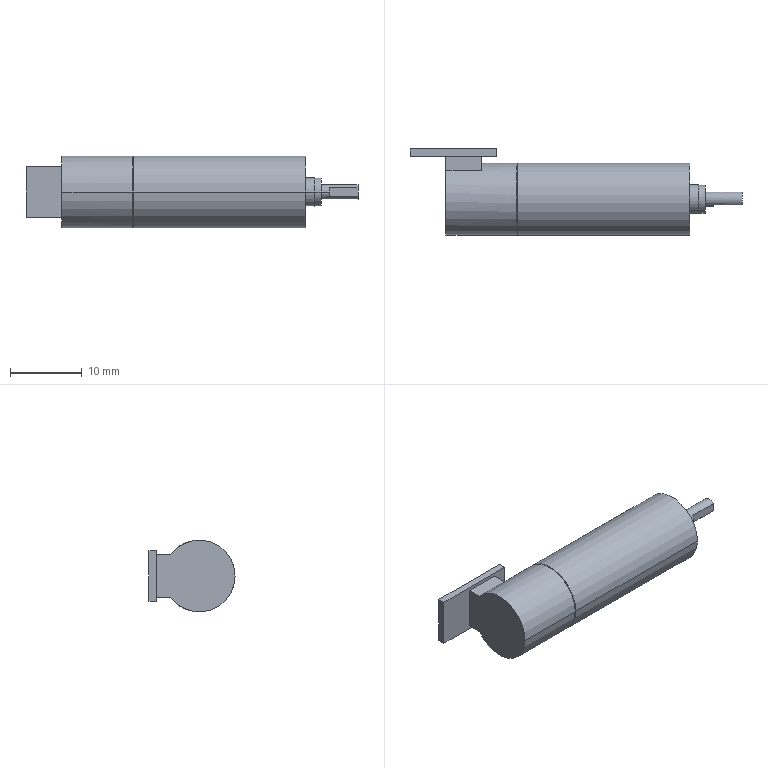Part | SolidWorks | features BaseBody 1 | 1 solid | 30 faces | box 46.3 x 12 x 10 mm | volume 2836 mm3 | plane 18 | cylinder 12 | commonest cylinder face diameters 10 x4 2 x2 3.9 x2 4 x2 9.8 x2
STEP:
#1=CARTESIAN_POINT('',(-31.3,5.,0.));
#2=VERTEX_POINT('',#1);
#3=CARTESIAN_POINT('',(-31.3,-5.,0.));
#4=VERTEX_POINT('',#3);
#5=CARTESIAN_POINT('',(-31.3,0.,0.));
#6=DIRECTION('',(1.,0.,0.));
#7=DIRECTION('',(0.,1.,0.));
#8=AXIS2_PLACEMENT_3D('',#5,#6,#7);
#9=CIRCLE('',#8,5.);
#10=EDGE_CURVE('',#2,#4,#9,.T.);
#11=ORIENTED_EDGE('',*,*,#10,.T.);
#12=CARTESIAN_POINT('',(-7.3,-5.,0.));
#13=VERTEX_POINT('',#12);
#14=CARTESIAN_POINT('',(0.,-5.,0.));
#15=DIRECTION('',(1.,0.,0.));
#16=VECTOR('',#15,1000.);
#17=LINE('',#14,#16);
#18=EDGE_CURVE('',#4,#13,#17,.T.);
#19=ORIENTED_EDGE('',*,*,#18,.T.);
#20=CARTESIAN_POINT('',(-7.3,5.,0.));
#21=VERTEX_POINT('',#20);
#22=CARTESIAN_POINT('',(-7.3,0.,0.));
#23=DIRECTION('',(-1.,0.,0.));
#24=DIRECTION('',(0.,1.,0.));
#25=AXIS2_PLACEMENT_3D('',#22,#23,#24);
#26=CIRCLE('',#25,5.);
#27=EDGE_CURVE('',#13,#21,#26,.T.);
#28=ORIENTED_EDGE('',*,*,#27,.T.);
#29=CARTESIAN_POINT('',(0.,5.,0.));
#30=DIRECTION('',(1.,0.,0.));
#31=VECTOR('',#30,1000.);
#32=LINE('',#29,#31);
#33=EDGE_CURVE('',#2,#21,#32,.T.);
#34=ORIENTED_EDGE('',*,*,#33,.F.);
#35=EDGE_LOOP('',(#11,#19,#28,#34));
#36=FACE_OUTER_BOUND('',#35,.T.);
#37=CARTESIAN_POINT('',(0.,0.,0.));
#38=DIRECTION('',(1.,0.,0.));
#39=DIRECTION('',(0.,1.,0.));
#40=AXIS2_PLACEMENT_3D('',#37,#38,#39);
#41=CYLINDRICAL_SURFACE('',#40,5.);
#42=ADVANCED_FACE('',(#36),#41,.T.);
#43=CARTESIAN_POINT('',(-7.3,-2.,0.));
#44=VERTEX_POINT('',#43);
#45=CARTESIAN_POINT('',(-7.3,2.,0.));
#46=VERTEX_POINT('',#45);
#47=CARTESIAN_POINT('',(-7.3,0.,0.));
#48=DIRECTION('',(-1.,0.,0.));
#49=DIRECTION('',(0.,1.,0.));
#50=AXIS2_PLACEMENT_3D('',#47,#48,#49);
#51=CIRCLE('',#50,2.);
#52=EDGE_CURVE('',#44,#46,#51,.T.);
#53=ORIENTED_EDGE('',*,*,#52,.F.);
#54=CARTESIAN_POINT('',(-6.02,-2.,0.));
#55=VERTEX_POINT('',#54);
#56=CARTESIAN_POINT('',(0.,-2.,0.));
#57=DIRECTION('',(1.,0.,0.));
#58=VECTOR('',#57,1000.);
#59=LINE('',#56,#58);
#60=EDGE_CURVE('',#44,#55,#59,.T.);
#61=ORIENTED_EDGE('',*,*,#60,.T.);
#62=CARTESIAN_POINT('',(-6.02,2.,0.));
#63=VERTEX_POINT('',#62);
#64=CARTESIAN_POINT('',(-6.02,0.,0.));
#65=DIRECTION('',(-1.,0.,0.));
#66=DIRECTION('',(0.,1.,0.));
#67=AXIS2_PLACEMENT_3D('',#64,#65,#66);
#68=CIRCLE('',#67,2.);
#69=EDGE_CURVE('',#55,#63,#68,.T.);
#70=ORIENTED_EDGE('',*,*,#69,.T.);
#71=CARTESIAN_POINT('',(0.,2.,0.));
#72=DIRECTION('',(1.,0.,0.));
#73=VECTOR('',#72,1000.);
#74=LINE('',#71,#73);
#75=EDGE_CURVE('',#46,#63,#74,.T.);
#76=ORIENTED_EDGE('',*,*,#75,.F.);
#77=EDGE_LOOP('',(#53,#61,#70,#76));
#78=FACE_OUTER_BOUND('',#77,.T.);
#79=CARTESIAN_POINT('',(0.,0.,0.));
#80=DIRECTION('',(1.,0.,0.));
#81=DIRECTION('',(0.,1.,0.));
#82=AXIS2_PLACEMENT_3D('',#79,#80,#81);
#83=CYLINDRICAL_SURFACE('',#82,2.);
#84=ADVANCED_FACE('',(#78),#83,.T.);
#85=CARTESIAN_POINT('',(-31.4,4.9,0.));
#86=VERTEX_POINT('',#85);
#87=CARTESIAN_POINT('',(-31.4,-4.9,0.));
#88=VERTEX_POINT('',#87);
#89=CARTESIAN_POINT('',(-31.4,0.,0.));
#90=DIRECTION('',(1.,0.,0.));
#91=DIRECTION('',(0.,1.,0.));
#92=AXIS2_PLACEMENT_3D('',#89,#90,#91);
#93=CIRCLE('',#92,4.9);
#94=EDGE_CURVE('',#86,#88,#93,.T.);
#95=ORIENTED_EDGE('',*,*,#94,.T.);
#96=CARTESIAN_POINT('',(-31.3,-4.9,0.));
#97=VERTEX_POINT('',#96);
#98=CARTESIAN_POINT('',(0.,-4.9,0.));
#99=DIRECTION('',(1.,0.,0.));
#100=VECTOR('',#99,1000.);
#101=LINE('',#98,#100);
#102=EDGE_CURVE('',#88,#97,#101,.T.);
#103=ORIENTED_EDGE('',*,*,#102,.T.);
#104=CARTESIAN_POINT('',(-31.3,4.9,0.));
#105=VERTEX_POINT('',#104);
#106=CARTESIAN_POINT('',(-31.3,0.,0.));
#107=DIRECTION('',(1.,0.,0.));
#108=DIRECTION('',(0.,1.,0.));
#109=AXIS2_PLACEMENT_3D('',#106,#107,#108);
#110=CIRCLE('',#109,4.9);
#111=EDGE_CURVE('',#105,#97,#110,.T.);
#112=ORIENTED_EDGE('',*,*,#111,.F.);
#113=CARTESIAN_POINT('',(0.,4.9,0.));
#114=DIRECTION('',(1.,0.,0.));
#115=VECTOR('',#114,1000.);
#116=LINE('',#113,#115);
#117=EDGE_CURVE('',#86,#105,#116,.T.);
#118=ORIENTED_EDGE('',*,*,#117,.F.);
#119=EDGE_LOOP('',(#95,#103,#112,#118));
#120=FACE_OUTER_BOUND('',#119,.T.);
#121=CARTESIAN_POINT('',(0.,0.,0.));
#122=DIRECTION('',(1.,0.,0.));
#123=DIRECTION('',(0.,1.,0.));
#124=AXIS2_PLACEMENT_3D('',#121,#122,#123);
#125=CYLINDRICAL_SURFACE('',#124,4.9);
#126=ADVANCED_FACE('',(#120),#125,.T.);
#127=CARTESIAN_POINT('',(-6.02,-1.95,0.));
#128=VERTEX_POINT('',#127);
#129=CARTESIAN_POINT('',(-6.02,1.95,0.));
#130=VERTEX_POINT('',#129);
#131=CARTESIAN_POINT('',(-6.02,0.,0.));
#132=DIRECTION('',(-1.,0.,0.));
#133=DIRECTION('',(0.,1.,0.));
#134=AXIS2_PLACEMENT_3D('',#131,#132,#133);
#135=CIRCLE('',#134,1.95);
#136=EDGE_CURVE('',#128,#130,#135,.T.);
#137=ORIENTED_EDGE('',*,*,#136,.F.);
#138=CARTESIAN_POINT('',(-5.14,-1.95,0.));
#139=VERTEX_POINT('',#138);
#140=CARTESIAN_POINT('',(0.,-1.95,0.));
#141=DIRECTION('',(1.,0.,0.));
#142=VECTOR('',#141,1000.);
#143=LINE('',#140,#142);
#144=EDGE_CURVE('',#128,#139,#143,.T.);
#145=ORIENTED_EDGE('',*,*,#144,.T.);
#146=CARTESIAN_POINT('',(-5.14,1.95,0.));
#147=VERTEX_POINT('',#146);
#148=CARTESIAN_POINT('',(-5.14,0.,0.));
#149=DIRECTION('',(-1.,0.,0.));
#150=DIRECTION('',(0.,1.,0.));
#151=AXIS2_PLACEMENT_3D('',#148,#149,#150);
#152=CIRCLE('',#151,1.95);
#153=EDGE_CURVE('',#139,#147,#152,.T.);
#154=ORIENTED_EDGE('',*,*,#153,.T.);
#155=CARTESIAN_POINT('',(0.,1.95,0.));
#156=DIRECTION('',(1.,0.,0.));
#157=VECTOR('',#156,1000.);
#158=LINE('',#155,#157);
#159=EDGE_CURVE('',#130,#147,#158,.T.);
#160=ORIENTED_EDGE('',*,*,#159,.F.);
#161=EDGE_LOOP('',(#137,#145,#154,#160));
#162=FACE_OUTER_BOUND('',#161,.T.);
#163=CARTESIAN_POINT('',(0.,0.,0.));
#164=DIRECTION('',(1.,0.,0.));
#165=DIRECTION('',(0.,1.,0.));
#166=AXIS2_PLACEMENT_3D('',#163,#164,#165);
#167=CYLINDRICAL_SURFACE('',#166,1.95);
#168=ADVANCED_FACE('',(#162),#167,.T.);
#169=CARTESIAN_POINT('',(-41.3,4.,3.));
#170=VERTEX_POINT('',#169);
#171=CARTESIAN_POINT('',(-41.3,-5.,0.));
#172=VERTEX_POINT('',#171);
#173=CARTESIAN_POINT('',(-41.3,0.,0.));
#174=DIRECTION('',(1.,0.,0.));
#175=DIRECTION('',(0.,1.,0.));
#176=AXIS2_PLACEMENT_3D('',#173,#174,#175);
#177=CIRCLE('',#176,5.);
#178=EDGE_CURVE('',#170,#172,#177,.T.);
#179=ORIENTED_EDGE('',*,*,#178,.T.);
#180=CARTESIAN_POINT('',(-31.4,-5.,0.));
#181=VERTEX_POINT('',#180);
#182=CARTESIAN_POINT('',(0.,-5.,0.));
#183=DIRECTION('',(1.,0.,0.));
#184=VECTOR('',#183,1000.);
#185=LINE('',#182,#184);
#186=EDGE_CURVE('',#172,#181,#185,.T.);
#187=ORIENTED_EDGE('',*,*,#186,.T.);
#188=CARTESIAN_POINT('',(-31.4,5.,0.));
#189=VERTEX_POINT('',#188);
#190=CARTESIAN_POINT('',(-31.4,0.,0.));
#191=DIRECTION('',(1.,0.,0.));
#192=DIRECTION('',(0.,1.,0.));
#193=AXIS2_PLACEMENT_3D('',#190,#191,#192);
#194=CIRCLE('',#193,5.);
#195=EDGE_CURVE('',#189,#181,#194,.T.);
#196=ORIENTED_EDGE('',*,*,#195,.F.);
#197=CARTESIAN_POINT('',(-36.3,5.,0.));
#198=VERTEX_POINT('',#197);
#199=CARTESIAN_POINT('',(0.,5.,0.));
#200=DIRECTION('',(1.,0.,0.));
#201=VECTOR('',#200,1000.);
#202=LINE('',#199,#201);
#203=EDGE_CURVE('',#198,#189,#202,.T.);
#204=ORIENTED_EDGE('',*,*,#203,.F.);
#205=CARTESIAN_POINT('',(-36.3,4.,3.));
#206=VERTEX_POINT('',#205);
#207=CARTESIAN_POINT('',(-36.3,0.,0.));
#208=DIRECTION('',(1.,0.,0.));
#209=DIRECTION('',(0.,1.,0.));
#210=AXIS2_PLACEMENT_3D('',#207,#208,#209);
#211=CIRCLE('',#210,5.);
#212=EDGE_CURVE('',#198,#206,#211,.T.);
#213=ORIENTED_EDGE('',*,*,#212,.T.);
#214=CARTESIAN_POINT('',(0.,4.,3.));
#215=DIRECTION('',(-1.,0.,0.));
#216=VECTOR('',#215,1000.);
#217=LINE('',#214,#216);
#218=EDGE_CURVE('',#206,#170,#217,.T.);
#219=ORIENTED_EDGE('',*,*,#218,.T.);
#220=EDGE_LOOP('',(#179,#187,#196,#204,#213,#219));
#221=FACE_OUTER_BOUND('',#220,.T.);
#222=CARTESIAN_POINT('',(0.,0.,0.));
#223=DIRECTION('',(1.,0.,0.));
#224=DIRECTION('',(0.,1.,0.));
#225=AXIS2_PLACEMENT_3D('',#222,#223,#224);
#226=CYLINDRICAL_SURFACE('',#225,5.);
#227=ADVANCED_FACE('',(#221),#226,.T.);
#228=CARTESIAN_POINT('',(-5.14,-1.,0.));
#229=VERTEX_POINT('',#228);
#230=CARTESIAN_POINT('',(-5.14,1.,0.));
#231=VERTEX_POINT('',#230);
#232=CARTESIAN_POINT('',(-5.14,0.,0.));
#233=DIRECTION('',(-1.,0.,0.));
#234=DIRECTION('',(0.,1.,0.));
#235=AXIS2_PLACEMENT_3D('',#232,#233,#234);
#236=CIRCLE('',#235,1.);
#237=EDGE_CURVE('',#229,#231,#236,.T.);
#238=ORIENTED_EDGE('',*,*,#237,.F.);
#239=CARTESIAN_POINT('',(-4.,-1.,0.));
#240=VERTEX_POINT('',#239);
#241=CARTESIAN_POINT('',(0.,-1.,0.));
#242=DIRECTION('',(1.,0.,0.));
#243=VECTOR('',#242,1000.);
#244=LINE('',#241,#243);
#245=EDGE_CURVE('',#229,#240,#244,.T.);
#246=ORIENTED_EDGE('',*,*,#245,.T.);
#247=CARTESIAN_POINT('',(-4.,-0.8,0.6));
#248=VERTEX_POINT('',#247);
#249=CARTESIAN_POINT('',(-4.,0.,0.));
#250=DIRECTION('',(-1.,0.,0.));
#251=DIRECTION('',(0.,1.,0.));
#252=AXIS2_PLACEMENT_3D('',#249,#250,#251);
#253=CIRCLE('',#252,1.);
#254=EDGE_CURVE('',#240,#248,#253,.T.);
#255=ORIENTED_EDGE('',*,*,#254,.T.);
#256=CARTESIAN_POINT('',(0.,-0.8,0.6));
#257=VERTEX_POINT('',#256);
#258=CARTESIAN_POINT('',(0.,-0.8,0.6));
#259=DIRECTION('',(1.,0.,0.));
#260=VECTOR('',#259,1000.);
#261=LINE('',#258,#260);
#262=EDGE_CURVE('',#248,#257,#261,.T.);
#263=ORIENTED_EDGE('',*,*,#262,.T.);
#264=CARTESIAN_POINT('',(0.,1.,0.));
#265=VERTEX_POINT('',#264);
#266=CARTESIAN_POINT('',(0.,0.,0.));
#267=DIRECTION('',(-1.,0.,0.));
#268=DIRECTION('',(0.,1.,0.));
#269=AXIS2_PLACEMENT_3D('',#266,#267,#268);
#270=CIRCLE('',#269,1.);
#271=EDGE_CURVE('',#257,#265,#270,.T.);
#272=ORIENTED_EDGE('',*,*,#271,.T.);
#273=CARTESIAN_POINT('',(0.,1.,0.));
#274=DIRECTION('',(1.,0.,0.));
#275=VECTOR('',#274,1000.);
#276=LINE('',#273,#275);
#277=EDGE_CURVE('',#231,#265,#276,.T.);
#278=ORIENTED_EDGE('',*,*,#277,.F.);
#279=EDGE_LOOP('',(#238,#246,#255,#263,#272,#278));
#280=FACE_OUTER_BOUND('',#279,.T.);
#281=CARTESIAN_POINT('',(0.,0.,0.));
#282=DIRECTION('',(1.,0.,0.));
#283=DIRECTION('',(0.,1.,0.));
#284=AXIS2_PLACEMENT_3D('',#281,#282,#283);
#285=CYLINDRICAL_SURFACE('',#284,1.);
#286=ADVANCED_FACE('',(#280),#285,.T.);
#287=ORIENTED_EDGE('',*,*,#18,.F.);
#288=CARTESIAN_POINT('',(-31.3,0.,0.));
#289=DIRECTION('',(1.,0.,0.));
#290=DIRECTION('',(0.,1.,0.));
#291=AXIS2_PLACEMENT_3D('',#288,#289,#290);
#292=CIRCLE('',#291,5.);
#293=EDGE_CURVE('',#4,#2,#292,.T.);
#294=ORIENTED_EDGE('',*,*,#293,.T.);
#295=ORIENTED_EDGE('',*,*,#33,.T.);
#296=CARTESIAN_POINT('',(-7.3,0.,0.));
#297=DIRECTION('',(-1.,0.,0.));
#298=DIRECTION('',(0.,1.,0.));
#299=AXIS2_PLACEMENT_3D('',#296,#297,#298);
#300=CIRCLE('',#299,5.);
#301=EDGE_CURVE('',#21,#13,#300,.T.);
#302=ORIENTED_EDGE('',*,*,#301,.T.);
#303=EDGE_LOOP('',(#287,#294,#295,#302));
#304=FACE_OUTER_BOUND('',#303,.T.);
#305=CARTESIAN_POINT('',(0.,0.,0.));
#306=DIRECTION('',(1.,0.,0.));
#307=DIRECTION('',(0.,1.,0.));
#308=AXIS2_PLACEMENT_3D('',#305,#306,#307);
#309=CYLINDRICAL_SURFACE('',#308,5.);
#310=ADVANCED_FACE('',(#304),#309,.T.);
#311=CARTESIAN_POINT('',(-7.3,0.,0.));
#312=DIRECTION('',(-1.,0.,0.));
#313=DIRECTION('',(0.,1.,0.));
#314=AXIS2_PLACEMENT_3D('',#311,#312,#313);
#315=CIRCLE('',#314,2.);
#316=EDGE_CURVE('',#46,#44,#315,.T.);
#317=ORIENTED_EDGE('',*,*,#316,.T.);
#318=ORIENTED_EDGE('',*,*,#52,.T.);
#319=EDGE_LOOP('',(#317,#318));
#320=FACE_BOUND('',#319,.T.);
#321=ORIENTED_EDGE('',*,*,#301,.F.);
#322=ORIENTED_EDGE('',*,*,#27,.F.);
#323=EDGE_LOOP('',(#321,#322));
#324=FACE_OUTER_BOUND('',#323,.T.);
#325=CARTESIAN_POINT('',(-7.3,2.,0.));
#326=DIRECTION('',(1.,0.,0.));
#327=DIRECTION('',(0.,1.,0.));
#328=AXIS2_PLACEMENT_3D('',#325,#326,#327);
#329=PLANE('',#328);
#330=ADVANCED_FACE('',(#320,#324),#329,.T.);
#331=ORIENTED_EDGE('',*,*,#10,.F.);
#332=ORIENTED_EDGE('',*,*,#293,.F.);
#333=EDGE_LOOP('',(#331,#332));
#334=FACE_OUTER_BOUND('',#333,.T.);
#335=ORIENTED_EDGE('',*,*,#111,.T.);
#336=CARTESIAN_POINT('',(-31.3,0.,0.));
#337=DIRECTION('',(1.,0.,0.));
#338=DIRECTION('',(0.,1.,0.));
#339=AXIS2_PLACEMENT_3D('',#336,#337,#338);
#340=CIRCLE('',#339,4.9);
#341=EDGE_CURVE('',#97,#105,#340,.T.);
#342=ORIENTED_EDGE('',*,*,#341,.T.);
#343=EDGE_LOOP('',(#335,#342));
#344=FACE_BOUND('',#343,.T.);
#345=CARTESIAN_POINT('',(-31.3,4.9,0.));
#346=DIRECTION('',(-1.,0.,0.));
#347=DIRECTION('',(0.,-1.,0.));
#348=AXIS2_PLACEMENT_3D('',#345,#346,#347);
#349=PLANE('',#348);
#350=ADVANCED_FACE('',(#334,#344),#349,.T.);
#351=ORIENTED_EDGE('',*,*,#60,.F.);
#352=ORIENTED_EDGE('',*,*,#316,.F.);
#353=ORIENTED_EDGE('',*,*,#75,.T.);
#354=CARTESIAN_POINT('',(-6.02,0.,0.));
#355=DIRECTION('',(-1.,0.,0.));
#356=DIRECTION('',(0.,1.,0.));
#357=AXIS2_PLACEMENT_3D('',#354,#355,#356);
#358=CIRCLE('',#357,2.);
#359=EDGE_CURVE('',#63,#55,#358,.T.);
#360=ORIENTED_EDGE('',*,*,#359,.T.);
#361=EDGE_LOOP('',(#351,#352,#353,#360));
#362=FACE_OUTER_BOUND('',#361,.T.);
#363=CARTESIAN_POINT('',(0.,0.,0.));
#364=DIRECTION('',(1.,0.,0.));
#365=DIRECTION('',(0.,1.,0.));
#366=AXIS2_PLACEMENT_3D('',#363,#364,#365);
#367=CYLINDRICAL_SURFACE('',#366,2.);
#368=ADVANCED_FACE('',(#362),#367,.T.);
#369=ORIENTED_EDGE('',*,*,#102,.F.);
#370=CARTESIAN_POINT('',(-31.4,0.,0.));
#371=DIRECTION('',(1.,0.,0.));
#372=DIRECTION('',(0.,1.,0.));
#373=AXIS2_PLACEMENT_3D('',#370,#371,#372);
#374=CIRCLE('',#373,4.9);
#375=EDGE_CURVE('',#88,#86,#374,.T.);
#376=ORIENTED_EDGE('',*,*,#375,.T.);
#377=ORIENTED_EDGE('',*,*,#117,.T.);
#378=ORIENTED_EDGE('',*,*,#341,.F.);
#379=EDGE_LOOP('',(#369,#376,#377,#378));
#380=FACE_OUTER_BOUND('',#379,.T.);
#381=CARTESIAN_POINT('',(0.,0.,0.));
#382=DIRECTION('',(1.,0.,0.));
#383=DIRECTION('',(0.,1.,0.));
#384=AXIS2_PLACEMENT_3D('',#381,#382,#383);
#385=CYLINDRICAL_SURFACE('',#384,4.9);
#386=ADVANCED_FACE('',(#380),#385,.T.);
#387=CARTESIAN_POINT('',(-6.02,0.,0.));
#388=DIRECTION('',(-1.,0.,0.));
#389=DIRECTION('',(0.,1.,0.));
#390=AXIS2_PLACEMENT_3D('',#387,#388,#389);
#391=CIRCLE('',#390,1.95);
#392=EDGE_CURVE('',#130,#128,#391,.T.);
#393=ORIENTED_EDGE('',*,*,#392,.T.);
#394=ORIENTED_EDGE('',*,*,#136,.T.);
#395=EDGE_LOOP('',(#393,#394));
#396=FACE_BOUND('',#395,.T.);
#397=ORIENTED_EDGE('',*,*,#359,.F.);
#398=ORIENTED_EDGE('',*,*,#69,.F.);
#399=EDGE_LOOP('',(#397,#398));
#400=FACE_OUTER_BOUND('',#399,.T.);
#401=CARTESIAN_POINT('',(-6.02,1.95,0.));
#402=DIRECTION('',(1.,0.,0.));
#403=DIRECTION('',(0.,1.,0.));
#404=AXIS2_PLACEMENT_3D('',#401,#402,#403);
#405=PLANE('',#404);
#406=ADVANCED_FACE('',(#396,#400),#405,.T.);
#407=ORIENTED_EDGE('',*,*,#94,.F.);
#408=ORIENTED_EDGE('',*,*,#375,.F.);
#409=EDGE_LOOP('',(#407,#408));
#410=FACE_BOUND('',#409,.T.);
#411=ORIENTED_EDGE('',*,*,#195,.T.);
#412=CARTESIAN_POINT('',(-31.4,0.,0.));
#413=DIRECTION('',(1.,0.,0.));
#414=DIRECTION('',(0.,1.,0.));
#415=AXIS2_PLACEMENT_3D('',#412,#413,#414);
#416=CIRCLE('',#415,5.);
#417=EDGE_CURVE('',#181,#189,#416,.T.);
#418=ORIENTED_EDGE('',*,*,#417,.T.);
#419=EDGE_LOOP('',(#411,#418));
#420=FACE_OUTER_BOUND('',#419,.T.);
#421=CARTESIAN_POINT('',(-31.4,5.,0.));
#422=DIRECTION('',(1.,0.,0.));
#423=DIRECTION('',(0.,1.,0.));
#424=AXIS2_PLACEMENT_3D('',#421,#422,#423);
#425=PLANE('',#424);
#426=ADVANCED_FACE('',(#410,#420),#425,.T.);
#427=ORIENTED_EDGE('',*,*,#144,.F.);
#428=ORIENTED_EDGE('',*,*,#392,.F.);
#429=ORIENTED_EDGE('',*,*,#159,.T.);
#430=CARTESIAN_POINT('',(-5.14,0.,0.));
#431=DIRECTION('',(-1.,0.,0.));
#432=DIRECTION('',(0.,1.,0.));
#433=AXIS2_PLACEMENT_3D('',#430,#431,#432);
#434=CIRCLE('',#433,1.95);
#435=EDGE_CURVE('',#147,#139,#434,.T.);
#436=ORIENTED_EDGE('',*,*,#435,.T.);
#437=EDGE_LOOP('',(#427,#428,#429,#436));
#438=FACE_OUTER_BOUND('',#437,.T.);
#439=CARTESIAN_POINT('',(0.,0.,0.));
#440=DIRECTION('',(1.,0.,0.));
#441=DIRECTION('',(0.,1.,0.));
#442=AXIS2_PLACEMENT_3D('',#439,#440,#441);
#443=CYLINDRICAL_SURFACE('',#442,1.95);
#444=ADVANCED_FACE('',(#438),#443,.T.);
#445=ORIENTED_EDGE('',*,*,#186,.F.);
#446=CARTESIAN_POINT('',(-41.3,4.,-3.));
#447=VERTEX_POINT('',#446);
#448=CARTESIAN_POINT('',(-41.3,0.,0.));
#449=DIRECTION('',(1.,0.,0.));
#450=DIRECTION('',(0.,1.,0.));
#451=AXIS2_PLACEMENT_3D('',#448,#449,#450);
#452=CIRCLE('',#451,5.);
#453=EDGE_CURVE('',#172,#447,#452,.T.);
#454=ORIENTED_EDGE('',*,*,#453,.T.);
#455=CARTESIAN_POINT('',(-36.3,4.,-3.));
#456=VERTEX_POINT('',#455);
#457=CARTESIAN_POINT('',(0.,4.,-3.));
#458=DIRECTION('',(1.,0.,0.));
#459=VECTOR('',#458,1000.);
#460=LINE('',#457,#459);
#461=EDGE_CURVE('',#447,#456,#460,.T.);
#462=ORIENTED_EDGE('',*,*,#461,.T.);
#463=CARTESIAN_POINT('',(-36.3,0.,0.));
#464=DIRECTION('',(1.,0.,0.));
#465=DIRECTION('',(0.,1.,0.));
#466=AXIS2_PLACEMENT_3D('',#463,#464,#465);
#467=CIRCLE('',#466,5.);
#468=EDGE_CURVE('',#456,#198,#467,.T.);
#469=ORIENTED_EDGE('',*,*,#468,.T.);
#470=ORIENTED_EDGE('',*,*,#203,.T.);
#471=ORIENTED_EDGE('',*,*,#417,.F.);
#472=EDGE_LOOP('',(#445,#454,#462,#469,#470,#471));
#473=FACE_OUTER_BOUND('',#472,.T.);
#474=CARTESIAN_POINT('',(0.,0.,0.));
#475=DIRECTION('',(1.,0.,0.));
#476=DIRECTION('',(0.,1.,0.));
#477=AXIS2_PLACEMENT_3D('',#474,#475,#476);
#478=CYLINDRICAL_SURFACE('',#477,5.);
#479=ADVANCED_FACE('',(#473),#478,.T.);
#480=CARTESIAN_POINT('',(-5.14,0.,0.));
#481=DIRECTION('',(-1.,0.,0.));
#482=DIRECTION('',(0.,1.,0.));
#483=AXIS2_PLACEMENT_3D('',#480,#481,#482);
#484=CIRCLE('',#483,1.);
#485=EDGE_CURVE('',#231,#229,#484,.T.);
#486=ORIENTED_EDGE('',*,*,#485,.T.);
#487=ORIENTED_EDGE('',*,*,#237,.T.);
#488=EDGE_LOOP('',(#486,#487));
#489=FACE_BOUND('',#488,.T.);
#490=ORIENTED_EDGE('',*,*,#435,.F.);
#491=ORIENTED_EDGE('',*,*,#153,.F.);
#492=EDGE_LOOP('',(#490,#491));
#493=FACE_OUTER_BOUND('',#492,.T.);
#494=CARTESIAN_POINT('',(-5.14,1.,0.));
#495=DIRECTION('',(1.,0.,0.));
#496=DIRECTION('',(0.,1.,0.));
#497=AXIS2_PLACEMENT_3D('',#494,#495,#496);
#498=PLANE('',#497);
#499=ADVANCED_FACE('',(#489,#493),#498,.T.);
#500=ORIENTED_EDGE('',*,*,#468,.F.);
#501=CARTESIAN_POINT('',(-36.3,6.,-3.));
#502=VERTEX_POINT('',#501);
#503=CARTESIAN_POINT('',(-36.3,0.,-3.));
#504=DIRECTION('',(0.,-1.,0.));
#505=VECTOR('',#504,1000.);
#506=LINE('',#503,#505);
#507=EDGE_CURVE('',#502,#456,#506,.T.);
#508=ORIENTED_EDGE('',*,*,#507,.F.);
#509=CARTESIAN_POINT('',(-36.3,6.,3.));
#510=VERTEX_POINT('',#509);
#511=CARTESIAN_POINT('',(-36.3,6.,0.));
#512=DIRECTION('',(0.,0.,-1.));
#513=VECTOR('',#512,1000.);
#514=LINE('',#511,#513);
#515=EDGE_CURVE('',#510,#502,#514,.T.);
#516=ORIENTED_EDGE('',*,*,#515,.F.);
#517=CARTESIAN_POINT('',(-36.3,0.,3.));
#518=DIRECTION('',(0.,1.,0.));
#519=VECTOR('',#518,1000.);
#520=LINE('',#517,#519);
#521=EDGE_CURVE('',#206,#510,#520,.T.);
#522=ORIENTED_EDGE('',*,*,#521,.F.);
#523=ORIENTED_EDGE('',*,*,#212,.F.);
#524=EDGE_LOOP('',(#500,#508,#516,#522,#523));
#525=FACE_OUTER_BOUND('',#524,.T.);
#526=CARTESIAN_POINT('',(-36.3,0.,0.));
#527=DIRECTION('',(-1.,0.,0.));
#528=DIRECTION('',(0.,0.,1.));
#529=AXIS2_PLACEMENT_3D('',#526,#527,#528);
#530=PLANE('',#529);
#531=ADVANCED_FACE('',(#525),#530,.F.);
#532=ORIENTED_EDGE('',*,*,#507,.T.);
#533=ORIENTED_EDGE('',*,*,#461,.F.);
#534=CARTESIAN_POINT('',(-41.3,6.,-3.));
#535=VERTEX_POINT('',#534);
#536=CARTESIAN_POINT('',(-41.3,0.,-3.));
#537=DIRECTION('',(0.,1.,0.));
#538=VECTOR('',#537,1000.);
#539=LINE('',#536,#538);
#540=EDGE_CURVE('',#447,#535,#539,.T.);
#541=ORIENTED_EDGE('',*,*,#540,.T.);
#542=CARTESIAN_POINT('',(-36.3,6.,-3.));
#543=DIRECTION('',(1.,0.,0.));
#544=VECTOR('',#543,1000.);
#545=LINE('',#542,#544);
#546=EDGE_CURVE('',#535,#502,#545,.T.);
#547=ORIENTED_EDGE('',*,*,#546,.T.);
#548=EDGE_LOOP('',(#532,#533,#541,#547));
#549=FACE_OUTER_BOUND('',#548,.T.);
#550=CARTESIAN_POINT('',(-36.3,0.,-3.));
#551=DIRECTION('',(0.,0.,-1.));
#552=DIRECTION('',(-1.,0.,0.));
#553=AXIS2_PLACEMENT_3D('',#550,#551,#552);
#554=PLANE('',#553);
#555=ADVANCED_FACE('',(#549),#554,.T.);
#556=ORIENTED_EDGE('',*,*,#540,.F.);
#557=ORIENTED_EDGE('',*,*,#453,.F.);
#558=ORIENTED_EDGE('',*,*,#178,.F.);
#559=CARTESIAN_POINT('',(-41.3,6.,3.));
#560=VERTEX_POINT('',#559);
#561=CARTESIAN_POINT('',(-41.3,5.,3.));
#562=DIRECTION('',(0.,1.,0.));
#563=VECTOR('',#562,1000.);
#564=LINE('',#561,#563);
#565=EDGE_CURVE('',#170,#560,#564,.T.);
#566=ORIENTED_EDGE('',*,*,#565,.T.);
#567=CARTESIAN_POINT('',(-41.3,6.,0.));
#568=DIRECTION('',(0.,0.,-1.));
#569=VECTOR('',#568,1000.);
#570=LINE('',#567,#569);
#571=EDGE_CURVE('',#560,#535,#570,.T.);
#572=ORIENTED_EDGE('',*,*,#571,.T.);
#573=EDGE_LOOP('',(#556,#557,#558,#566,#572));
#574=FACE_OUTER_BOUND('',#573,.T.);
#575=CARTESIAN_POINT('',(-41.3,5.,0.));
#576=DIRECTION('',(-1.,0.,0.));
#577=DIRECTION('',(0.,-1.,0.));
#578=AXIS2_PLACEMENT_3D('',#575,#576,#577);
#579=PLANE('',#578);
#580=ADVANCED_FACE('',(#574),#579,.T.);
#581=ORIENTED_EDGE('',*,*,#218,.F.);
#582=ORIENTED_EDGE('',*,*,#521,.T.);
#583=CARTESIAN_POINT('',(-36.3,6.,3.));
#584=DIRECTION('',(1.,0.,0.));
#585=VECTOR('',#584,1000.);
#586=LINE('',#583,#585);
#587=EDGE_CURVE('',#560,#510,#586,.T.);
#588=ORIENTED_EDGE('',*,*,#587,.F.);
#589=ORIENTED_EDGE('',*,*,#565,.F.);
#590=EDGE_LOOP('',(#581,#582,#588,#589));
#591=FACE_OUTER_BOUND('',#590,.T.);
#592=CARTESIAN_POINT('',(-36.3,0.,3.));
#593=DIRECTION('',(0.,0.,-1.));
#594=DIRECTION('',(0.,1.,0.));
#595=AXIS2_PLACEMENT_3D('',#592,#593,#594);
#596=PLANE('',#595);
#597=ADVANCED_FACE('',(#591),#596,.F.);
#598=ORIENTED_EDGE('',*,*,#245,.F.);
#599=ORIENTED_EDGE('',*,*,#485,.F.);
#600=ORIENTED_EDGE('',*,*,#277,.T.);
#601=CARTESIAN_POINT('',(0.,-0.8,-0.6));
#602=VERTEX_POINT('',#601);
#603=CARTESIAN_POINT('',(0.,0.,0.));
#604=DIRECTION('',(-1.,0.,0.));
#605=DIRECTION('',(0.,1.,0.));
#606=AXIS2_PLACEMENT_3D('',#603,#604,#605);
#607=CIRCLE('',#606,1.);
#608=EDGE_CURVE('',#265,#602,#607,.T.);
#609=ORIENTED_EDGE('',*,*,#608,.T.);
#610=CARTESIAN_POINT('',(-4.,-0.8,-0.6));
#611=VERTEX_POINT('',#610);
#612=CARTESIAN_POINT('',(0.,-0.8,-0.6));
#613=DIRECTION('',(-1.,0.,0.));
#614=VECTOR('',#613,1000.);
#615=LINE('',#612,#614);
#616=EDGE_CURVE('',#602,#611,#615,.T.);
#617=ORIENTED_EDGE('',*,*,#616,.T.);
#618=CARTESIAN_POINT('',(-4.,0.,0.));
#619=DIRECTION('',(-1.,0.,0.));
#620=DIRECTION('',(0.,1.,0.));
#621=AXIS2_PLACEMENT_3D('',#618,#619,#620);
#622=CIRCLE('',#621,1.);
#623=EDGE_CURVE('',#611,#240,#622,.T.);
#624=ORIENTED_EDGE('',*,*,#623,.T.);
#625=EDGE_LOOP('',(#598,#599,#600,#609,#617,#624));
#626=FACE_OUTER_BOUND('',#625,.T.);
#627=CARTESIAN_POINT('',(0.,0.,0.));
#628=DIRECTION('',(1.,0.,0.));
#629=DIRECTION('',(0.,1.,0.));
#630=AXIS2_PLACEMENT_3D('',#627,#628,#629);
#631=CYLINDRICAL_SURFACE('',#630,1.);
#632=ADVANCED_FACE('',(#626),#631,.T.);
#633=CARTESIAN_POINT('',(-46.3,6.,-3.5));
#634=VERTEX_POINT('',#633);
#635=CARTESIAN_POINT('',(-34.3,6.,-3.5));
#636=VERTEX_POINT('',#635);
#637=CARTESIAN_POINT('',(-34.3,6.,-3.5));
#638=DIRECTION('',(1.,0.,0.));
#639=VECTOR('',#638,1000.);
#640=LINE('',#637,#639);
#641=EDGE_CURVE('',#634,#636,#640,.T.);
#642=ORIENTED_EDGE('',*,*,#641,.T.);
#643=CARTESIAN_POINT('',(-34.3,6.,3.5));
#644=VERTEX_POINT('',#643);
#645=CARTESIAN_POINT('',(-34.3,6.,-3.5));
#646=DIRECTION('',(0.,0.,1.));
#647=VECTOR('',#646,1000.);
#648=LINE('',#645,#647);
#649=EDGE_CURVE('',#636,#644,#648,.T.);
#650=ORIENTED_EDGE('',*,*,#649,.T.);
#651=CARTESIAN_POINT('',(-46.3,6.,3.5));
#652=VERTEX_POINT('',#651);
#653=CARTESIAN_POINT('',(-34.3,6.,3.5));
#654=DIRECTION('',(-1.,0.,0.));
#655=VECTOR('',#654,1000.);
#656=LINE('',#653,#655);
#657=EDGE_CURVE('',#644,#652,#656,.T.);
#658=ORIENTED_EDGE('',*,*,#657,.T.);
#659=CARTESIAN_POINT('',(-46.3,6.,-3.5));
#660=DIRECTION('',(0.,0.,-1.));
#661=VECTOR('',#660,1000.);
#662=LINE('',#659,#661);
#663=EDGE_CURVE('',#652,#634,#662,.T.);
#664=ORIENTED_EDGE('',*,*,#663,.T.);
#665=EDGE_LOOP('',(#642,#650,#658,#664));
#666=FACE_OUTER_BOUND('',#665,.T.);
#667=ORIENTED_EDGE('',*,*,#587,.T.);
#668=ORIENTED_EDGE('',*,*,#515,.T.);
#669=ORIENTED_EDGE('',*,*,#546,.F.);
#670=ORIENTED_EDGE('',*,*,#571,.F.);
#671=EDGE_LOOP('',(#667,#668,#669,#670));
#672=FACE_BOUND('',#671,.T.);
#673=CARTESIAN_POINT('',(-34.3,6.,-3.5));
#674=DIRECTION('',(0.,-1.,0.));
#675=DIRECTION('',(1.,0.,0.));
#676=AXIS2_PLACEMENT_3D('',#673,#674,#675);
#677=PLANE('',#676);
#678=ADVANCED_FACE('',(#666,#672),#677,.T.);
#679=CARTESIAN_POINT('',(-4.,-0.8,0.));
#680=DIRECTION('',(0.,0.,1.));
#681=VECTOR('',#680,1000.);
#682=LINE('',#679,#681);
#683=EDGE_CURVE('',#611,#248,#682,.T.);
#684=ORIENTED_EDGE('',*,*,#683,.T.);
#685=ORIENTED_EDGE('',*,*,#254,.F.);
#686=ORIENTED_EDGE('',*,*,#623,.F.);
#687=EDGE_LOOP('',(#684,#685,#686));
#688=FACE_OUTER_BOUND('',#687,.T.);
#689=CARTESIAN_POINT('',(-4.,0.,0.));
#690=DIRECTION('',(1.,0.,0.));
#691=DIRECTION('',(0.,1.,0.));
#692=AXIS2_PLACEMENT_3D('',#689,#690,#691);
#693=PLANE('',#692);
#694=ADVANCED_FACE('',(#688),#693,.T.);
#695=ORIENTED_EDGE('',*,*,#683,.F.);
#696=ORIENTED_EDGE('',*,*,#616,.F.);
#697=CARTESIAN_POINT('',(0.,-0.8,0.));
#698=DIRECTION('',(0.,0.,1.));
#699=VECTOR('',#698,1000.);
#700=LINE('',#697,#699);
#701=EDGE_CURVE('',#602,#257,#700,.T.);
#702=ORIENTED_EDGE('',*,*,#701,.T.);
#703=ORIENTED_EDGE('',*,*,#262,.F.);
#704=EDGE_LOOP('',(#695,#696,#702,#703));
#705=FACE_OUTER_BOUND('',#704,.T.);
#706=CARTESIAN_POINT('',(-4.,-0.8,0.));
#707=DIRECTION('',(0.,-1.,0.));
#708=DIRECTION('',(1.,0.,0.));
#709=AXIS2_PLACEMENT_3D('',#706,#707,#708);
#710=PLANE('',#709);
#711=ADVANCED_FACE('',(#705),#710,.T.);
#712=ORIENTED_EDGE('',*,*,#271,.F.);
#713=ORIENTED_EDGE('',*,*,#701,.F.);
#714=ORIENTED_EDGE('',*,*,#608,.F.);
#715=EDGE_LOOP('',(#712,#713,#714));
#716=FACE_OUTER_BOUND('',#715,.T.);
#717=CARTESIAN_POINT('',(0.,0.,0.));
#718=DIRECTION('',(1.,0.,0.));
#719=DIRECTION('',(0.,1.,0.));
#720=AXIS2_PLACEMENT_3D('',#717,#718,#719);
#721=PLANE('',#720);
#722=ADVANCED_FACE('',(#716),#721,.T.);
#723=ORIENTED_EDGE('',*,*,#649,.F.);
#724=CARTESIAN_POINT('',(-34.3,7.,-3.5));
#725=VERTEX_POINT('',#724);
#726=CARTESIAN_POINT('',(-34.3,0.,-3.5));
#727=DIRECTION('',(0.,-1.,0.));
#728=VECTOR('',#727,1000.);
#729=LINE('',#726,#728);
#730=EDGE_CURVE('',#725,#636,#729,.T.);
#731=ORIENTED_EDGE('',*,*,#730,.F.);
#732=CARTESIAN_POINT('',(-34.3,7.,3.5));
#733=VERTEX_POINT('',#732);
#734=CARTESIAN_POINT('',(-34.3,7.,0.));
#735=DIRECTION('',(0.,0.,-1.));
#736=VECTOR('',#735,1000.);
#737=LINE('',#734,#736);
#738=EDGE_CURVE('',#733,#725,#737,.T.);
#739=ORIENTED_EDGE('',*,*,#738,.F.);
#740=CARTESIAN_POINT('',(-34.3,0.,3.5));
#741=DIRECTION('',(0.,1.,0.));
#742=VECTOR('',#741,1000.);
#743=LINE('',#740,#742);
#744=EDGE_CURVE('',#644,#733,#743,.T.);
#745=ORIENTED_EDGE('',*,*,#744,.F.);
#746=EDGE_LOOP('',(#723,#731,#739,#745));
#747=FACE_OUTER_BOUND('',#746,.T.);
#748=CARTESIAN_POINT('',(-34.3,0.,0.));
#749=DIRECTION('',(-1.,0.,0.));
#750=DIRECTION('',(0.,0.,1.));
#751=AXIS2_PLACEMENT_3D('',#748,#749,#750);
#752=PLANE('',#751);
#753=ADVANCED_FACE('',(#747),#752,.F.);
#754=CARTESIAN_POINT('',(-46.3,7.,-3.5));
#755=VERTEX_POINT('',#754);
#756=CARTESIAN_POINT('',(-34.3,7.,-3.5));
#757=DIRECTION('',(1.,0.,0.));
#758=VECTOR('',#757,1000.);
#759=LINE('',#756,#758);
#760=EDGE_CURVE('',#755,#725,#759,.T.);
#761=ORIENTED_EDGE('',*,*,#760,.T.);
#762=ORIENTED_EDGE('',*,*,#730,.T.);
#763=ORIENTED_EDGE('',*,*,#641,.F.);
#764=CARTESIAN_POINT('',(-46.3,7.,-3.5));
#765=DIRECTION('',(0.,1.,0.));
#766=VECTOR('',#765,1000.);
#767=LINE('',#764,#766);
#768=EDGE_CURVE('',#634,#755,#767,.T.);
#769=ORIENTED_EDGE('',*,*,#768,.T.);
#770=EDGE_LOOP('',(#761,#762,#763,#769));
#771=FACE_OUTER_BOUND('',#770,.T.);
#772=CARTESIAN_POINT('',(-34.3,7.,-3.5));
#773=DIRECTION('',(0.,0.,-1.));
#774=DIRECTION('',(0.,1.,0.));
#775=AXIS2_PLACEMENT_3D('',#772,#773,#774);
#776=PLANE('',#775);
#777=ADVANCED_FACE('',(#771),#776,.T.);
#778=ORIENTED_EDGE('',*,*,#768,.F.);
#779=ORIENTED_EDGE('',*,*,#663,.F.);
#780=CARTESIAN_POINT('',(-46.3,7.,3.5));
#781=VERTEX_POINT('',#780);
#782=CARTESIAN_POINT('',(-46.3,0.,3.5));
#783=DIRECTION('',(0.,1.,0.));
#784=VECTOR('',#783,1000.);
#785=LINE('',#782,#784);
#786=EDGE_CURVE('',#652,#781,#785,.T.);
#787=ORIENTED_EDGE('',*,*,#786,.T.);
#788=CARTESIAN_POINT('',(-46.3,7.,0.));
#789=DIRECTION('',(0.,0.,-1.));
#790=VECTOR('',#789,1000.);
#791=LINE('',#788,#790);
#792=EDGE_CURVE('',#781,#755,#791,.T.);
#793=ORIENTED_EDGE('',*,*,#792,.T.);
#794=EDGE_LOOP('',(#778,#779,#787,#793));
#795=FACE_OUTER_BOUND('',#794,.T.);
#796=CARTESIAN_POINT('',(-46.3,0.,0.));
#797=DIRECTION('',(-1.,0.,0.));
#798=DIRECTION('',(0.,0.,1.));
#799=AXIS2_PLACEMENT_3D('',#796,#797,#798);
#800=PLANE('',#799);
#801=ADVANCED_FACE('',(#795),#800,.T.);
#802=ORIENTED_EDGE('',*,*,#657,.F.);
#803=ORIENTED_EDGE('',*,*,#744,.T.);
#804=CARTESIAN_POINT('',(-34.3,7.,3.5));
#805=DIRECTION('',(-1.,0.,0.));
#806=VECTOR('',#805,1000.);
#807=LINE('',#804,#806);
#808=EDGE_CURVE('',#733,#781,#807,.T.);
#809=ORIENTED_EDGE('',*,*,#808,.T.);
#810=ORIENTED_EDGE('',*,*,#786,.F.);
#811=EDGE_LOOP('',(#802,#803,#809,#810));
#812=FACE_OUTER_BOUND('',#811,.T.);
#813=CARTESIAN_POINT('',(-34.3,7.,3.5));
#814=DIRECTION('',(0.,0.,1.));
#815=DIRECTION('',(1.,0.,0.));
#816=AXIS2_PLACEMENT_3D('',#813,#814,#815);
#817=PLANE('',#816);
#818=ADVANCED_FACE('',(#812),#817,.T.);
#819=ORIENTED_EDGE('',*,*,#808,.F.);
#820=ORIENTED_EDGE('',*,*,#738,.T.);
#821=ORIENTED_EDGE('',*,*,#760,.F.);
#822=ORIENTED_EDGE('',*,*,#792,.F.);
#823=EDGE_LOOP('',(#819,#820,#821,#822));
#824=FACE_OUTER_BOUND('',#823,.T.);
#825=CARTESIAN_POINT('',(-34.3,7.,-3.5));
#826=DIRECTION('',(0.,1.,0.));
#827=DIRECTION('',(-1.,0.,0.));
#828=AXIS2_PLACEMENT_3D('',#825,#826,#827);
#829=PLANE('',#828);
#830=ADVANCED_FACE('',(#824),#829,.T.);
#831=CLOSED_SHELL('',(#42,#84,#126,#168,#227,#286,#310,#330,#350,#368,#386,#406,#426,#444,#479,#499,#531,#555,#580,#597,#632,#678,#694,#711,#722,#753,#777,#801,#818,#830));
#832=MANIFOLD_SOLID_BREP('',#831);
#833=CARTESIAN_POINT('',(0.,0.,0.));
#834=DIRECTION('',(0.,0.,1.));
#835=DIRECTION('',(1.,0.,0.));
#836=AXIS2_PLACEMENT_3D('',#833,#834,#835);
#837=(LENGTH_UNIT()NAMED_UNIT(*)SI_UNIT(.MILLI.,.METRE.));
#838=UNCERTAINTY_MEASURE_WITH_UNIT(LENGTH_MEASURE(0.00001),#837,'','');
#839=(NAMED_UNIT(*)PLANE_ANGLE_UNIT()SI_UNIT($,.RADIAN.));
#840=(NAMED_UNIT(*)SI_UNIT($,.STERADIAN.)SOLID_ANGLE_UNIT());
#841=(GEOMETRIC_REPRESENTATION_CONTEXT(3)GLOBAL_UNCERTAINTY_ASSIGNED_CONTEXT((#838))GLOBAL_UNIT_ASSIGNED_CONTEXT((#837,#839,#840))REPRESENTATION_CONTEXT('',''));
#842=ADVANCED_BREP_SHAPE_REPRESENTATION('',(#832,#836),#841);